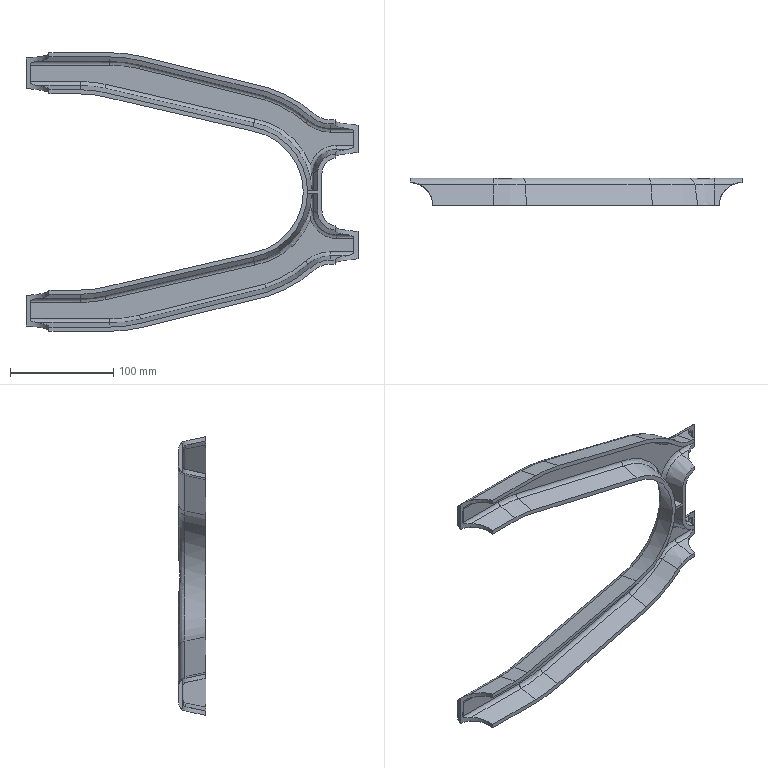Part | SolidWorks | features VarFillet 12, Fillet 2, BaseBody 1 | 1 solid | 132 faces | box 321.75 x 26.25 x 270 mm | volume 200467 mm3 | plane 47 | spline 33 | cylinder 30 | cone 11 | torus 11 | commonest cylinder face diameters 8 x14 16 x12 44.5 x4